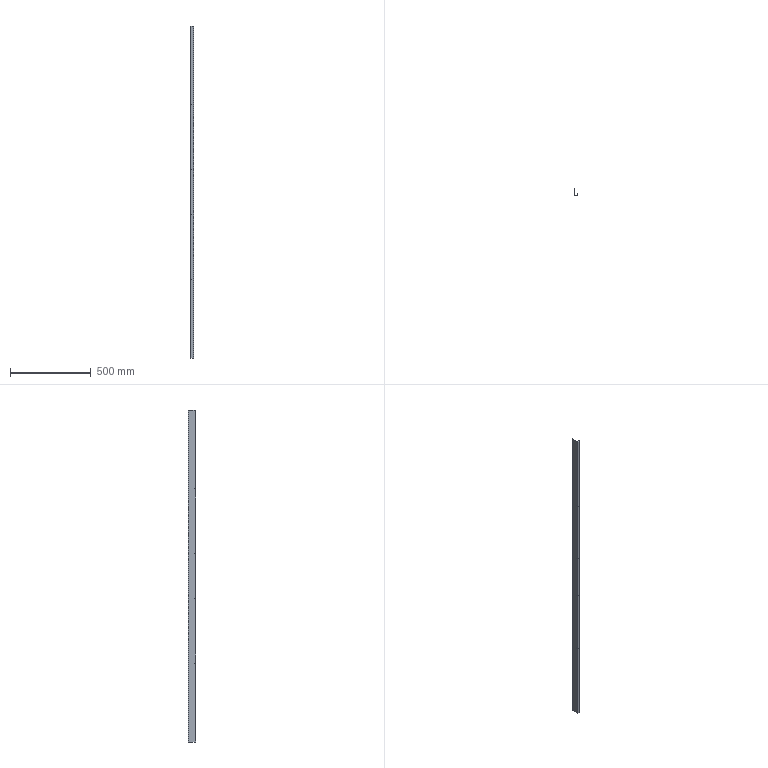Part | 1 solid | 62 faces | box 19 x 45 x 2056 mm | volume 214261 mm3 | plane 50 | cylinder 12 | commonest cylinder face diameters 2 x6 5 x6